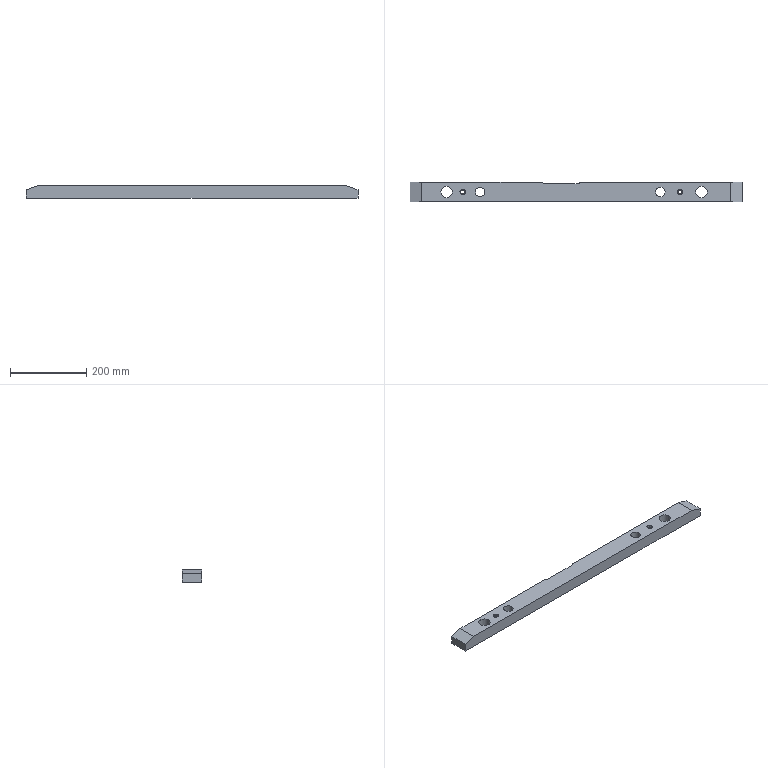Part | STEP file | gslz 2016.10.28-13_id494_x_t | 1 solid | 40 faces | box 870 x 50 x 32 mm | volume 1277939 mm3 | cylinder 20 | plane 10 | cone 10 | commonest cylinder face diameters 5.2 x4 6.8 x4 18 x4 10.3 x2 14 x2 25 x2